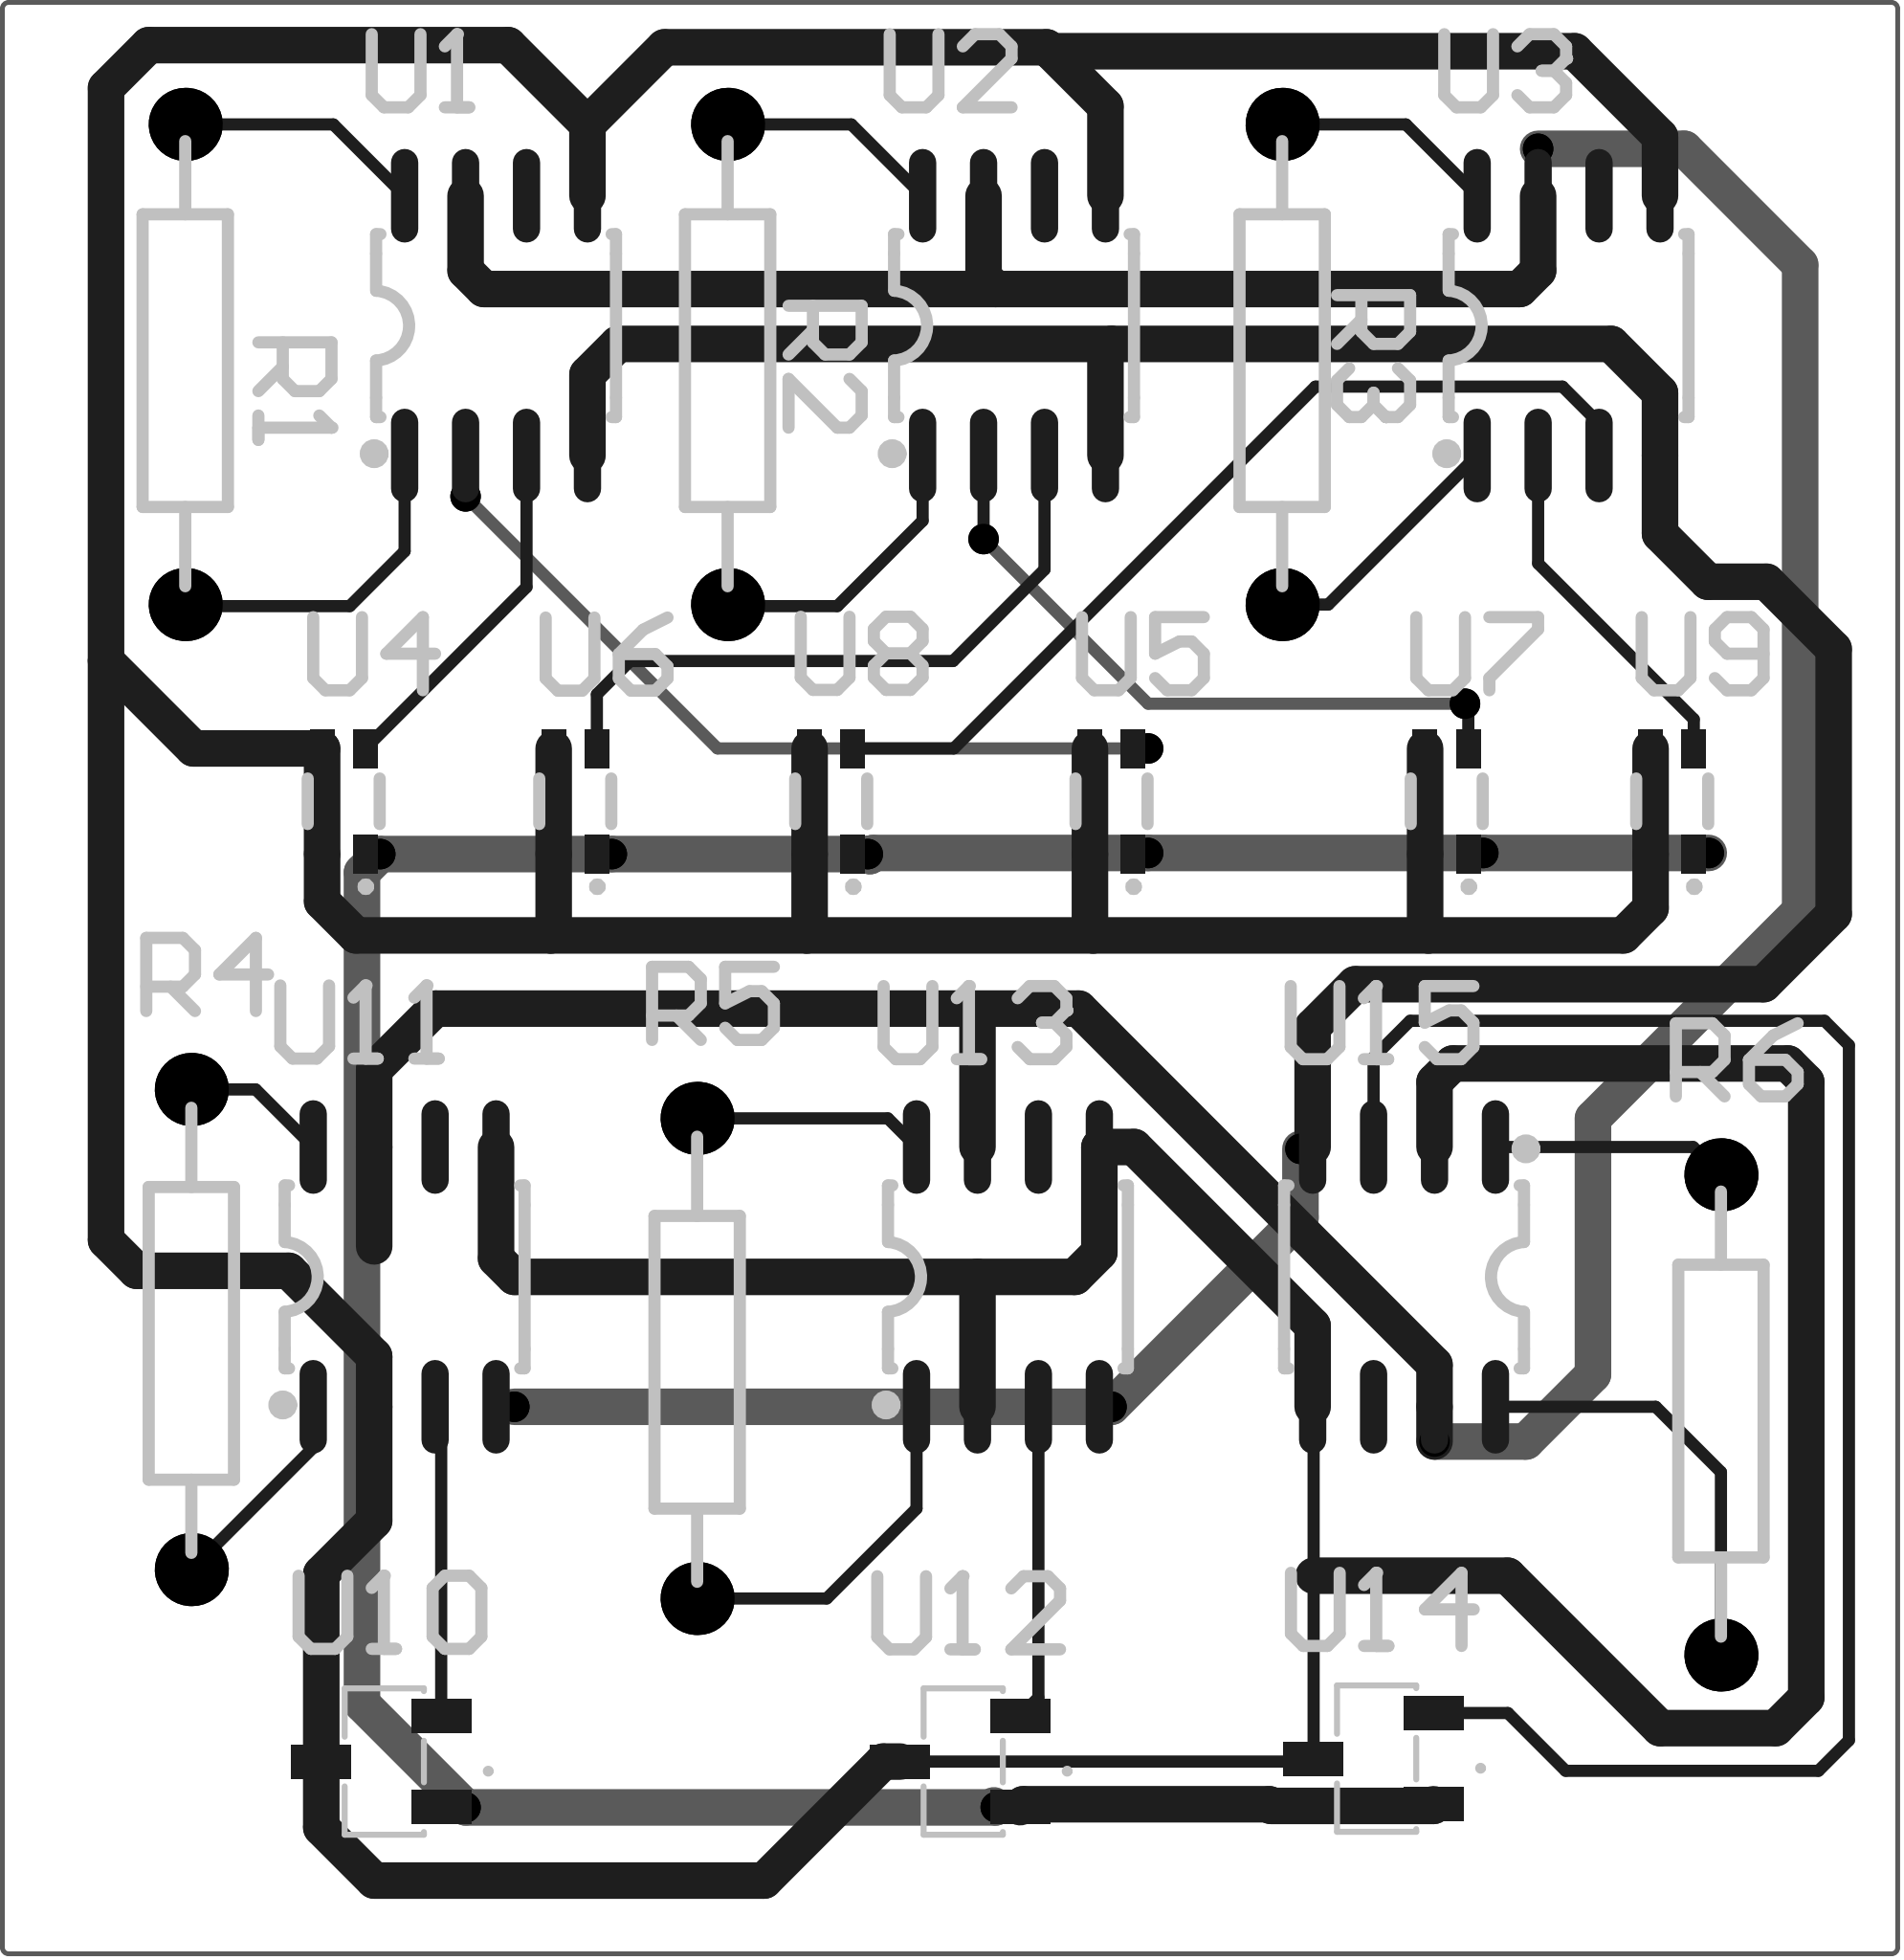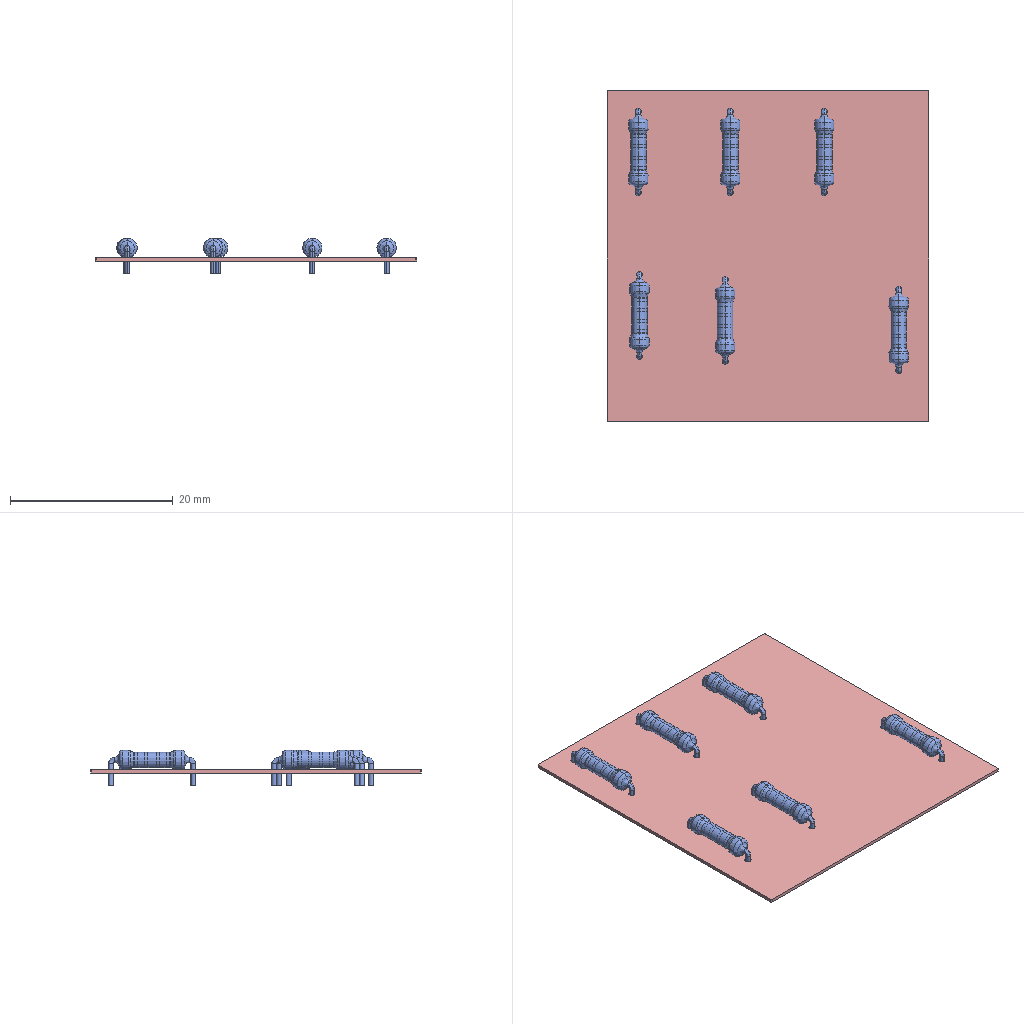Circuit board layout | Altium Designer | box 39.5 x 40.6 x 4.4 mm
Layer stack:
# Altium Designer layer stack of  (unit mm; dielectric type: 0 none, 1 core, 2 prepreg, 3 surface material)
index,name,kind,layer,copper_thickness_mm,dielectric_type,dielectric_thickness_mm,dielectric_material,dielectric_constant
0,Top Paste,other,,,,,,
1,Top Overlay,other,,,,,,
2,Top Solder,dielectric,,,3,0.0102,Solder Resist,3.5
3,Top Layer,copper,Top Layer,0.0356,,,,
4,Dielectric 1,dielectric,,,0,0.32,FR-4,4.8
5,Bottom Layer,copper,Bottom Layer,0.0356,,,,
6,Bottom Solder,dielectric,,,3,0.0102,Solder Resist,3.5
7,Bottom Overlay,other,,,,,,
8,Bottom Paste,other,,,,,,
# drill layer pairs: low layer,high layer
drill_pair,Top Layer,Bottom Layer
Part placement:
Designator,Comment,Layer,Footprint,Center-X(mm),Center-Y(mm),Rotation
R1,1K,TopLayer,R一般电阻/10mm,42.545,98.505,90
R2,1K,TopLayer,R一般电阻/10mm,53.848,98.505,90
R3,1K,TopLayer,R一般电阻/10mm,65.405,98.505,90
R4,5.5K,TopLayer,R一般电阻/10mm,42.672,78.406,270
R5,5.5K,TopLayer,R一般电阻/10mm,53.213,77.804,270
R6,5.5K,TopLayer,R一般电阻/10mm,74.549,76.628,90
U5,HG106A,TopLayer,SOP-4_L1.5-W1.5-P0.90-LS2.5-BL,61.849,89.408,90
U11,AD620ARZ-REEL,TopLayer,SOIC-8_L5.0-W4.0-P1.27-LS6.0-BL,47.117,79.502,0
U10,JSM3144,TopLayer,SOT-23-3_L2.9-W1.6-P1.90-LS2.8-BR-CW,46.629,69.408,0
U7,HG106A,TopLayer,SOP-4_L1.5-W1.5-P0.90-LS2.5-BL,68.834,89.408,90
U15,AD620ARZ-REEL,TopLayer,SOIC-8_L5.0-W4.0-P1.27-LS6.0-BL,67.945,79.502,180
U8,HG106A,TopLayer,SOP-4_L1.5-W1.5-P0.90-LS2.5-BL,56.007,89.408,90
U4,HG106A,TopLayer,SOP-4_L1.5-W1.5-P0.90-LS2.5-BL,45.847,89.408,90
U12,JSM3144,TopLayer,SOT-23-3_L2.9-W1.6-P1.90-LS2.8-BR-CW,58.694,69.408,0
U6,HG106A,TopLayer,SOP-4_L1.5-W1.5-P0.90-LS2.5-BL,50.673,89.408,90
U2,AD620ARZ-REEL,TopLayer,SOIC-8_L5.0-W4.0-P1.27-LS6.0-BL,59.817,99.314,0
U9,HG106A,TopLayer,SOP-4_L1.5-W1.5-P0.90-LS2.5-BL,73.533,89.408,90
U13,AD620ARZ-REEL,TopLayer,SOIC-8_L5.0-W4.0-P1.27-LS6.0-BL,59.69,79.502,0
U14,JSM3144,TopLayer,SOT-23-3_L2.9-W1.6-P1.90-LS2.8-BR-CW,67.31,69.469,0
U3,AD620ARZ-REEL,TopLayer,SOIC-8_L5.0-W4.0-P1.27-LS6.0-BL,71.374,99.314,0
U1,AD620ARZ-REEL,TopLayer,SOIC-8_L5.0-W4.0-P1.27-LS6.0-BL,49.022,99.314,0
Pad and via stacks:
# Altium Designer via and pad stacks of  (unit mm). Each distinct definition once, with the count of objects using it.
# via: kind,start_layer,end_layer,hole_mm,diameter_mm,mode(0 simple;1 top-mid-bottom;2 full stack),diameter_per_layer,count,example_net
# pad: kind,layer,hole_mm,hole_type(0 round;1 square;2 slot),plating,top_size,top_shape(1 round;2 rect;3 octagon;9 rounded rect),mid_size,bottom_size,mode,footprint,size_per_layer,count,example
pad,Multi-Layer,0.762,0,plated,1.524x1.524,1,1.524x1.524,1.524x1.524,0,R\u00D2\u00BB\u00B0\u00E3\u00B5\u00E7\u00D7\u00E8/10mm,,12,R2.1
pad,Top Layer,0,0,plated,0.5684x1.95,1,0.5684x1.95,0.5684x1.95,0,SOIC-8_L5.0-W4.0-P1.27-LS6.0-BL,,48,U15.5
pad,Top Layer,0,0,plated,0.7x1.25,2,0.7x1.25,0.7x1.25,0,SOT-23-3_L2.9-W1.6-P1.90-LS2.8-BR-CW,,9,U14.1
pad,Top Layer,0,0,plated,0.5x0.8,2,0.5x0.8,0.5x0.8,0,SOP-4_L1.5-W1.5-P0.90-LS2.5-BL,,24,U4.4
via,Top Layer,Bottom Layer,0.381,0.635,0,,17,+5
Design rules, without the lines most boards share:
# Altium Designer design rules of  (exported by Altium Designer, unit mm)
# columns: name | kind | enabled | priority | scope1 | scope2 | descriptor | typed fields (field=value)
Clearance | 0 | enabled | 1 | All | All | Clearance Constraint (Gap=10mil) (All),(All) | gap=0.254
PlaneConnect | 6 | enabled | 1 | All | All | Power Plane Connect Rule(Relief Connect )(Expansion=20mil) (Conductor Width=10mil) (Air Gap=10mil) (Entries=4) (All) | relief_conductor_width=0.254 relief_entries=4 relief_expansion=0.508
PolygonConnect | 20 | enabled | 1 | All | All | Polygon Connect Rule(Relief Connect )(Conductor Width=10mil) (Relief Angle=90 Angle) (Entries=4) (Air Gap Width=10mil) (All),(All) | connect_style(0=relief,1=direct,2=none)=0 relief_conductor_width=0.254 relief_entries=4
Width | 2 | enabled | 1 | All | All | Width Constraint (Min=10mil) (Max=222mil) (Preferred=10mil) (All) |
RoutingVias | 11 | enabled | 1 | All | All | Routing Via (MinHoleWidth=28mil) (MaxHoleWidth=28mil) (PreferredHoleWidth=28mil) (MinWidth=50mil) (MaxWidth=50mil) (PreferedWidth=50mil) (All) | via_min_hole=0.7112 via_max_hole=0.7112 via_preferred_diameter=1.27 via_preferred_hole=0.7112
PasteMaskExpansion | 14 | enabled | 1 | All | All | Paste Mask Expansion (Expansion =0mil) (All) | expansion=0
SolderMaskExpansion | 13 | enabled | 1 | All | All | Solder Mask Expansion (Expansion =4mil) (All) | expansion=0.1016
DiffPairsRouting | 51 | enabled | 1 | All | All | Differential Pairs Uncoupled Length using the Gap Constraints (Min=10mil) (Max=10mil) (Prefered=10mil)  and Width Constraints (Min=15mil) (Max=15mil) (Prefered=15mil) (All) |
HoleToHoleClearance | 52 | enabled | 1 | All | All | Hole To Hole Clearance (Gap=10mil) (All),(All) | gap=0.254
Classes set for this board:
# Altium Designer classes of  (member kind: 0 net, 1 component, 2 from-to, 3 pad, 4 layer, 5 differential pair, 6 design channel, 7 polygon, 8 structure, 9 xSignal)
# columns: class name | member kind | superclass | members
Sheet1 | 1 | no | R1; R2; R3; R4; R5; R6; U2; U3; U4; U5; U6; U7; U8; U9; U11; U12; U13; U14; U15; U3; U15; U12; U5; U1; U7; U9; U4; U14; U2; U10; U8; U13; U6; U11;